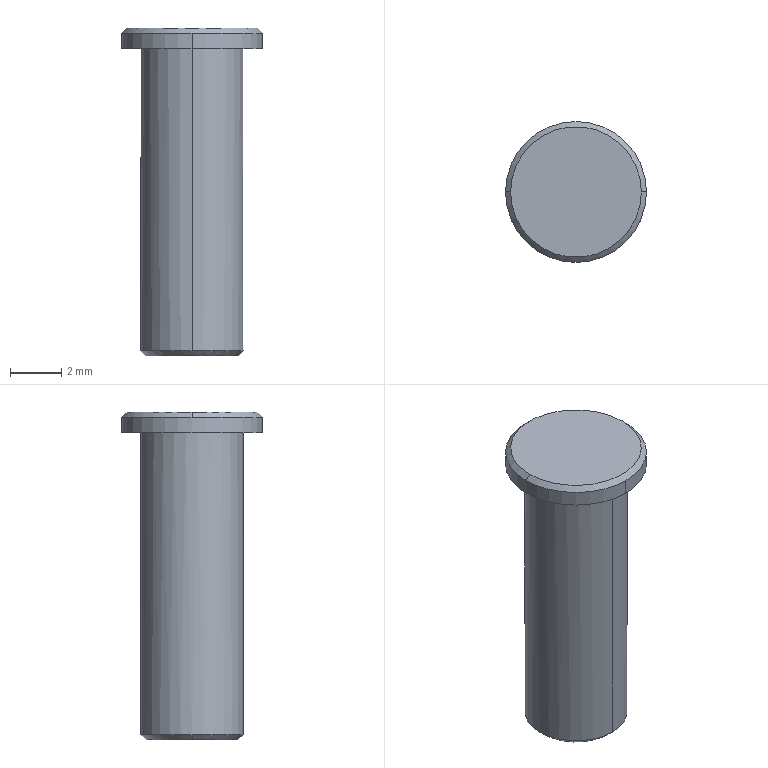Part | NX | 1 solid | 11 faces | box 5.5 x 5.5 x 12.8 mm | volume 169.223 mm3 | cylinder 4 | cone 4 | plane 3 | commonest cylinder face diameters 4 x2 5.5 x2
STEP:
#1=CARTESIAN_POINT('',(0.,2.75,0.));
#2=VERTEX_POINT('',#1);
#3=CARTESIAN_POINT('',(0.,-2.75,0.));
#4=VERTEX_POINT('',#3);
#5=CARTESIAN_POINT('',(0.,0.,0.));
#6=DIRECTION('',(0.,0.,1.));
#7=DIRECTION('',(0.,1.,0.));
#8=AXIS2_PLACEMENT_3D('',#5,#6,#7);
#9=CIRCLE('',#8,2.75);
#10=EDGE_CURVE('',#2,#4,#9,.T.);
#11=ORIENTED_EDGE('',*,*,#10,.F.);
#12=CARTESIAN_POINT('',(0.,0.,0.));
#13=DIRECTION('',(0.,0.,1.));
#14=DIRECTION('',(0.,1.,0.));
#15=AXIS2_PLACEMENT_3D('',#12,#13,#14);
#16=CIRCLE('',#15,2.75);
#17=EDGE_CURVE('',#4,#2,#16,.T.);
#18=ORIENTED_EDGE('',*,*,#17,.F.);
#19=EDGE_LOOP('',(#11,#18));
#20=FACE_BOUND('',#19,.T.);
#21=CARTESIAN_POINT('',(0.,2.,0.));
#22=VERTEX_POINT('',#21);
#23=CARTESIAN_POINT('',(0.,-2.,0.));
#24=VERTEX_POINT('',#23);
#25=CARTESIAN_POINT('',(0.,0.,0.));
#26=DIRECTION('',(0.,0.,-1.));
#27=DIRECTION('',(0.,1.,0.));
#28=AXIS2_PLACEMENT_3D('',#25,#26,#27);
#29=CIRCLE('',#28,2.);
#30=EDGE_CURVE('',#22,#24,#29,.T.);
#31=ORIENTED_EDGE('',*,*,#30,.F.);
#32=CARTESIAN_POINT('',(0.,0.,0.));
#33=DIRECTION('',(0.,0.,-1.));
#34=DIRECTION('',(0.,1.,0.));
#35=AXIS2_PLACEMENT_3D('',#32,#33,#34);
#36=CIRCLE('',#35,2.);
#37=EDGE_CURVE('',#24,#22,#36,.T.);
#38=ORIENTED_EDGE('',*,*,#37,.F.);
#39=EDGE_LOOP('',(#31,#38));
#40=FACE_BOUND('',#39,.T.);
#41=CARTESIAN_POINT('',(0.,0.,0.));
#42=DIRECTION('',(0.,0.,1.));
#43=DIRECTION('',(1.,0.,0.));
#44=AXIS2_PLACEMENT_3D('',#41,#42,#43);
#45=PLANE('',#44);
#46=ADVANCED_FACE('',(#20,#40),#45,.F.);
#47=ORIENTED_EDGE('',*,*,#10,.T.);
#48=CARTESIAN_POINT('',(0.,-2.75,0.6));
#49=VERTEX_POINT('',#48);
#50=CARTESIAN_POINT('',(0.,-2.75,0.));
#51=DIRECTION('',(0.,0.,1.));
#52=VECTOR('',#51,1000.);
#53=LINE('',#50,#52);
#54=EDGE_CURVE('',#49,#4,#53,.F.);
#55=ORIENTED_EDGE('',*,*,#54,.F.);
#56=CARTESIAN_POINT('',(-2.75,0.,0.6));
#57=VERTEX_POINT('',#56);
#58=CARTESIAN_POINT('',(0.,0.,0.6));
#59=DIRECTION('',(0.,0.,-1.));
#60=DIRECTION('',(-1.,0.,0.));
#61=AXIS2_PLACEMENT_3D('',#58,#59,#60);
#62=CIRCLE('',#61,2.75);
#63=EDGE_CURVE('',#49,#57,#62,.T.);
#64=ORIENTED_EDGE('',*,*,#63,.T.);
#65=CARTESIAN_POINT('',(0.,2.75,0.6));
#66=VERTEX_POINT('',#65);
#67=CARTESIAN_POINT('',(0.,0.,0.6));
#68=DIRECTION('',(0.,0.,-1.));
#69=DIRECTION('',(-1.,0.,0.));
#70=AXIS2_PLACEMENT_3D('',#67,#68,#69);
#71=CIRCLE('',#70,2.75);
#72=EDGE_CURVE('',#57,#66,#71,.T.);
#73=ORIENTED_EDGE('',*,*,#72,.T.);
#74=CARTESIAN_POINT('',(0.,2.75,0.));
#75=DIRECTION('',(0.,0.,1.));
#76=VECTOR('',#75,1000.);
#77=LINE('',#74,#76);
#78=EDGE_CURVE('',#66,#2,#77,.F.);
#79=ORIENTED_EDGE('',*,*,#78,.T.);
#80=EDGE_LOOP('',(#47,#55,#64,#73,#79));
#81=FACE_BOUND('',#80,.T.);
#82=CARTESIAN_POINT('',(0.,0.,0.));
#83=DIRECTION('',(0.,0.,1.));
#84=DIRECTION('',(0.,1.,0.));
#85=AXIS2_PLACEMENT_3D('',#82,#83,#84);
#86=CYLINDRICAL_SURFACE('',#85,2.75);
#87=ADVANCED_FACE('',(#81),#86,.T.);
#88=ORIENTED_EDGE('',*,*,#30,.T.);
#89=CARTESIAN_POINT('',(0.,-2.,-11.8));
#90=VERTEX_POINT('',#89);
#91=CARTESIAN_POINT('',(0.,-2.,0.));
#92=DIRECTION('',(0.,0.,-1.));
#93=VECTOR('',#92,1000.);
#94=LINE('',#91,#93);
#95=EDGE_CURVE('',#90,#24,#94,.F.);
#96=ORIENTED_EDGE('',*,*,#95,.F.);
#97=CARTESIAN_POINT('',(2.,0.,-11.8));
#98=VERTEX_POINT('',#97);
#99=CARTESIAN_POINT('',(0.,0.,-11.8));
#100=DIRECTION('',(0.,0.,1.));
#101=DIRECTION('',(1.,0.,0.));
#102=AXIS2_PLACEMENT_3D('',#99,#100,#101);
#103=CIRCLE('',#102,2.);
#104=EDGE_CURVE('',#90,#98,#103,.T.);
#105=ORIENTED_EDGE('',*,*,#104,.T.);
#106=CARTESIAN_POINT('',(0.,2.,-11.8));
#107=VERTEX_POINT('',#106);
#108=CARTESIAN_POINT('',(0.,0.,-11.8));
#109=DIRECTION('',(0.,0.,1.));
#110=DIRECTION('',(1.,0.,0.));
#111=AXIS2_PLACEMENT_3D('',#108,#109,#110);
#112=CIRCLE('',#111,2.);
#113=EDGE_CURVE('',#98,#107,#112,.T.);
#114=ORIENTED_EDGE('',*,*,#113,.T.);
#115=CARTESIAN_POINT('',(0.,2.,0.));
#116=DIRECTION('',(0.,0.,-1.));
#117=VECTOR('',#116,1000.);
#118=LINE('',#115,#117);
#119=EDGE_CURVE('',#107,#22,#118,.F.);
#120=ORIENTED_EDGE('',*,*,#119,.T.);
#121=EDGE_LOOP('',(#88,#96,#105,#114,#120));
#122=FACE_BOUND('',#121,.T.);
#123=CARTESIAN_POINT('',(0.,0.,0.));
#124=DIRECTION('',(0.,0.,-1.));
#125=DIRECTION('',(0.,-1.,0.));
#126=AXIS2_PLACEMENT_3D('',#123,#124,#125);
#127=CYLINDRICAL_SURFACE('',#126,2.);
#128=ADVANCED_FACE('',(#122),#127,.T.);
#129=CARTESIAN_POINT('',(1.8,0.,-12.));
#130=VERTEX_POINT('',#129);
#131=CARTESIAN_POINT('',(-1.8,0.,-12.));
#132=VERTEX_POINT('',#131);
#133=CARTESIAN_POINT('',(0.,0.,-12.));
#134=DIRECTION('',(0.,0.,1.));
#135=DIRECTION('',(1.,0.,0.));
#136=AXIS2_PLACEMENT_3D('',#133,#134,#135);
#137=CIRCLE('',#136,1.8);
#138=EDGE_CURVE('',#130,#132,#137,.T.);
#139=ORIENTED_EDGE('',*,*,#138,.F.);
#140=CARTESIAN_POINT('',(0.,0.,-12.));
#141=DIRECTION('',(0.,0.,1.));
#142=DIRECTION('',(1.,0.,0.));
#143=AXIS2_PLACEMENT_3D('',#140,#141,#142);
#144=CIRCLE('',#143,1.8);
#145=EDGE_CURVE('',#132,#130,#144,.T.);
#146=ORIENTED_EDGE('',*,*,#145,.F.);
#147=EDGE_LOOP('',(#139,#146));
#148=FACE_BOUND('',#147,.T.);
#149=CARTESIAN_POINT('',(0.,0.,-12.));
#150=DIRECTION('',(0.,0.,-1.));
#151=DIRECTION('',(0.,-1.,0.));
#152=AXIS2_PLACEMENT_3D('',#149,#150,#151);
#153=PLANE('',#152);
#154=ADVANCED_FACE('',(#148),#153,.T.);
#155=CARTESIAN_POINT('',(2.55,0.,0.8));
#156=VERTEX_POINT('',#155);
#157=CARTESIAN_POINT('',(-2.55,0.,0.8));
#158=VERTEX_POINT('',#157);
#159=CARTESIAN_POINT('',(0.,0.,0.8));
#160=DIRECTION('',(0.,0.,-1.));
#161=DIRECTION('',(-1.,0.,0.));
#162=AXIS2_PLACEMENT_3D('',#159,#160,#161);
#163=CIRCLE('',#162,2.55);
#164=EDGE_CURVE('',#156,#158,#163,.T.);
#165=ORIENTED_EDGE('',*,*,#164,.F.);
#166=CARTESIAN_POINT('',(0.,0.,0.8));
#167=DIRECTION('',(0.,0.,-1.));
#168=DIRECTION('',(-1.,0.,0.));
#169=AXIS2_PLACEMENT_3D('',#166,#167,#168);
#170=CIRCLE('',#169,2.55);
#171=EDGE_CURVE('',#158,#156,#170,.T.);
#172=ORIENTED_EDGE('',*,*,#171,.F.);
#173=EDGE_LOOP('',(#165,#172));
#174=FACE_BOUND('',#173,.T.);
#175=CARTESIAN_POINT('',(0.,0.,0.8));
#176=DIRECTION('',(0.,0.,1.));
#177=DIRECTION('',(1.,0.,0.));
#178=AXIS2_PLACEMENT_3D('',#175,#176,#177);
#179=PLANE('',#178);
#180=ADVANCED_FACE('',(#174),#179,.T.);
#181=ORIENTED_EDGE('',*,*,#63,.F.);
#182=CARTESIAN_POINT('',(2.75,0.,0.6));
#183=VERTEX_POINT('',#182);
#184=CARTESIAN_POINT('',(0.,0.,0.6));
#185=DIRECTION('',(0.,0.,-1.));
#186=DIRECTION('',(-1.,0.,0.));
#187=AXIS2_PLACEMENT_3D('',#184,#185,#186);
#188=CIRCLE('',#187,2.75);
#189=EDGE_CURVE('',#183,#49,#188,.T.);
#190=ORIENTED_EDGE('',*,*,#189,.F.);
#191=CARTESIAN_POINT('',(2.55,0.,0.8));
#192=DIRECTION('',(0.7071,0.,-0.7071));
#193=VECTOR('',#192,1000.);
#194=LINE('',#191,#193);
#195=EDGE_CURVE('',#183,#156,#194,.F.);
#196=ORIENTED_EDGE('',*,*,#195,.T.);
#197=ORIENTED_EDGE('',*,*,#164,.T.);
#198=CARTESIAN_POINT('',(-2.55,0.,0.8));
#199=DIRECTION('',(-0.7071,0.,-0.7071));
#200=VECTOR('',#199,1000.);
#201=LINE('',#198,#200);
#202=EDGE_CURVE('',#57,#158,#201,.F.);
#203=ORIENTED_EDGE('',*,*,#202,.F.);
#204=EDGE_LOOP('',(#181,#190,#196,#197,#203));
#205=FACE_BOUND('',#204,.T.);
#206=CARTESIAN_POINT('',(0.,0.,0.8));
#207=DIRECTION('',(0.,0.,-1.));
#208=DIRECTION('',(-1.,0.,0.));
#209=AXIS2_PLACEMENT_3D('',#206,#207,#208);
#210=CONICAL_SURFACE('',#209,2.55,0.7854);
#211=ADVANCED_FACE('',(#205),#210,.T.);
#212=CARTESIAN_POINT('',(-2.,0.,-11.8));
#213=VERTEX_POINT('',#212);
#214=CARTESIAN_POINT('',(0.,0.,-11.8));
#215=DIRECTION('',(0.,0.,1.));
#216=DIRECTION('',(1.,0.,0.));
#217=AXIS2_PLACEMENT_3D('',#214,#215,#216);
#218=CIRCLE('',#217,2.);
#219=EDGE_CURVE('',#107,#213,#218,.T.);
#220=ORIENTED_EDGE('',*,*,#219,.F.);
#221=ORIENTED_EDGE('',*,*,#113,.F.);
#222=CARTESIAN_POINT('',(2.,0.,-11.8));
#223=DIRECTION('',(0.7071,0.,0.7071));
#224=VECTOR('',#223,1000.);
#225=LINE('',#222,#224);
#226=EDGE_CURVE('',#130,#98,#225,.T.);
#227=ORIENTED_EDGE('',*,*,#226,.F.);
#228=ORIENTED_EDGE('',*,*,#138,.T.);
#229=CARTESIAN_POINT('',(-2.,0.,-11.8));
#230=DIRECTION('',(-0.7071,0.,0.7071));
#231=VECTOR('',#230,1000.);
#232=LINE('',#229,#231);
#233=EDGE_CURVE('',#132,#213,#232,.T.);
#234=ORIENTED_EDGE('',*,*,#233,.T.);
#235=EDGE_LOOP('',(#220,#221,#227,#228,#234));
#236=FACE_BOUND('',#235,.T.);
#237=CARTESIAN_POINT('',(0.,0.,-11.8));
#238=DIRECTION('',(0.,0.,1.));
#239=DIRECTION('',(1.,0.,0.));
#240=AXIS2_PLACEMENT_3D('',#237,#238,#239);
#241=CONICAL_SURFACE('',#240,2.,0.7854);
#242=ADVANCED_FACE('',(#236),#241,.T.);
#243=ORIENTED_EDGE('',*,*,#226,.T.);
#244=ORIENTED_EDGE('',*,*,#104,.F.);
#245=CARTESIAN_POINT('',(0.,0.,-11.8));
#246=DIRECTION('',(0.,0.,1.));
#247=DIRECTION('',(1.,0.,0.));
#248=AXIS2_PLACEMENT_3D('',#245,#246,#247);
#249=CIRCLE('',#248,2.);
#250=EDGE_CURVE('',#213,#90,#249,.T.);
#251=ORIENTED_EDGE('',*,*,#250,.F.);
#252=ORIENTED_EDGE('',*,*,#233,.F.);
#253=ORIENTED_EDGE('',*,*,#145,.T.);
#254=EDGE_LOOP('',(#243,#244,#251,#252,#253));
#255=FACE_BOUND('',#254,.T.);
#256=CARTESIAN_POINT('',(0.,0.,-11.8));
#257=DIRECTION('',(0.,0.,1.));
#258=DIRECTION('',(1.,0.,0.));
#259=AXIS2_PLACEMENT_3D('',#256,#257,#258);
#260=CONICAL_SURFACE('',#259,2.,0.7854);
#261=ADVANCED_FACE('',(#255),#260,.T.);
#262=ORIENTED_EDGE('',*,*,#219,.T.);
#263=ORIENTED_EDGE('',*,*,#250,.T.);
#264=ORIENTED_EDGE('',*,*,#95,.T.);
#265=ORIENTED_EDGE('',*,*,#37,.T.);
#266=ORIENTED_EDGE('',*,*,#119,.F.);
#267=EDGE_LOOP('',(#262,#263,#264,#265,#266));
#268=FACE_BOUND('',#267,.T.);
#269=CARTESIAN_POINT('',(0.,0.,0.));
#270=DIRECTION('',(0.,0.,-1.));
#271=DIRECTION('',(0.,-1.,0.));
#272=AXIS2_PLACEMENT_3D('',#269,#270,#271);
#273=CYLINDRICAL_SURFACE('',#272,2.);
#274=ADVANCED_FACE('',(#268),#273,.T.);
#275=ORIENTED_EDGE('',*,*,#202,.T.);
#276=ORIENTED_EDGE('',*,*,#171,.T.);
#277=ORIENTED_EDGE('',*,*,#195,.F.);
#278=CARTESIAN_POINT('',(0.,0.,0.6));
#279=DIRECTION('',(0.,0.,-1.));
#280=DIRECTION('',(-1.,0.,0.));
#281=AXIS2_PLACEMENT_3D('',#278,#279,#280);
#282=CIRCLE('',#281,2.75);
#283=EDGE_CURVE('',#66,#183,#282,.T.);
#284=ORIENTED_EDGE('',*,*,#283,.F.);
#285=ORIENTED_EDGE('',*,*,#72,.F.);
#286=EDGE_LOOP('',(#275,#276,#277,#284,#285));
#287=FACE_BOUND('',#286,.T.);
#288=CARTESIAN_POINT('',(0.,0.,0.8));
#289=DIRECTION('',(0.,0.,-1.));
#290=DIRECTION('',(-1.,0.,0.));
#291=AXIS2_PLACEMENT_3D('',#288,#289,#290);
#292=CONICAL_SURFACE('',#291,2.55,0.7854);
#293=ADVANCED_FACE('',(#287),#292,.T.);
#294=ORIENTED_EDGE('',*,*,#54,.T.);
#295=ORIENTED_EDGE('',*,*,#17,.T.);
#296=ORIENTED_EDGE('',*,*,#78,.F.);
#297=ORIENTED_EDGE('',*,*,#283,.T.);
#298=ORIENTED_EDGE('',*,*,#189,.T.);
#299=EDGE_LOOP('',(#294,#295,#296,#297,#298));
#300=FACE_BOUND('',#299,.T.);
#301=CARTESIAN_POINT('',(0.,0.,0.));
#302=DIRECTION('',(0.,0.,1.));
#303=DIRECTION('',(0.,1.,0.));
#304=AXIS2_PLACEMENT_3D('',#301,#302,#303);
#305=CYLINDRICAL_SURFACE('',#304,2.75);
#306=ADVANCED_FACE('',(#300),#305,.T.);
#307=CLOSED_SHELL('',(#46,#87,#128,#154,#180,#211,#242,#261,#274,#293,#306));
#308=MANIFOLD_SOLID_BREP('',#307);
#309=(LENGTH_UNIT()NAMED_UNIT(*)SI_UNIT(.MILLI.,.METRE.));
#310=UNCERTAINTY_MEASURE_WITH_UNIT(LENGTH_MEASURE(0.00001),#309,'','');
#311=(NAMED_UNIT(*)PLANE_ANGLE_UNIT()SI_UNIT($,.RADIAN.));
#312=(NAMED_UNIT(*)SI_UNIT($,.STERADIAN.)SOLID_ANGLE_UNIT());
#313=(GEOMETRIC_REPRESENTATION_CONTEXT(3)GLOBAL_UNCERTAINTY_ASSIGNED_CONTEXT((#310))GLOBAL_UNIT_ASSIGNED_CONTEXT((#309,#311,#312))REPRESENTATION_CONTEXT('',''));
#314=ADVANCED_BREP_SHAPE_REPRESENTATION('',(#308),#313);